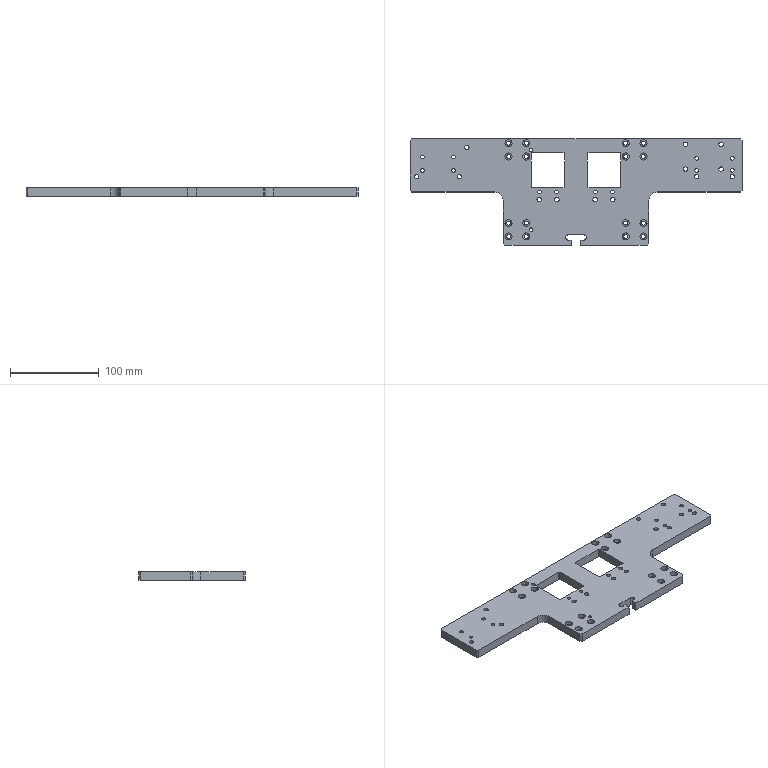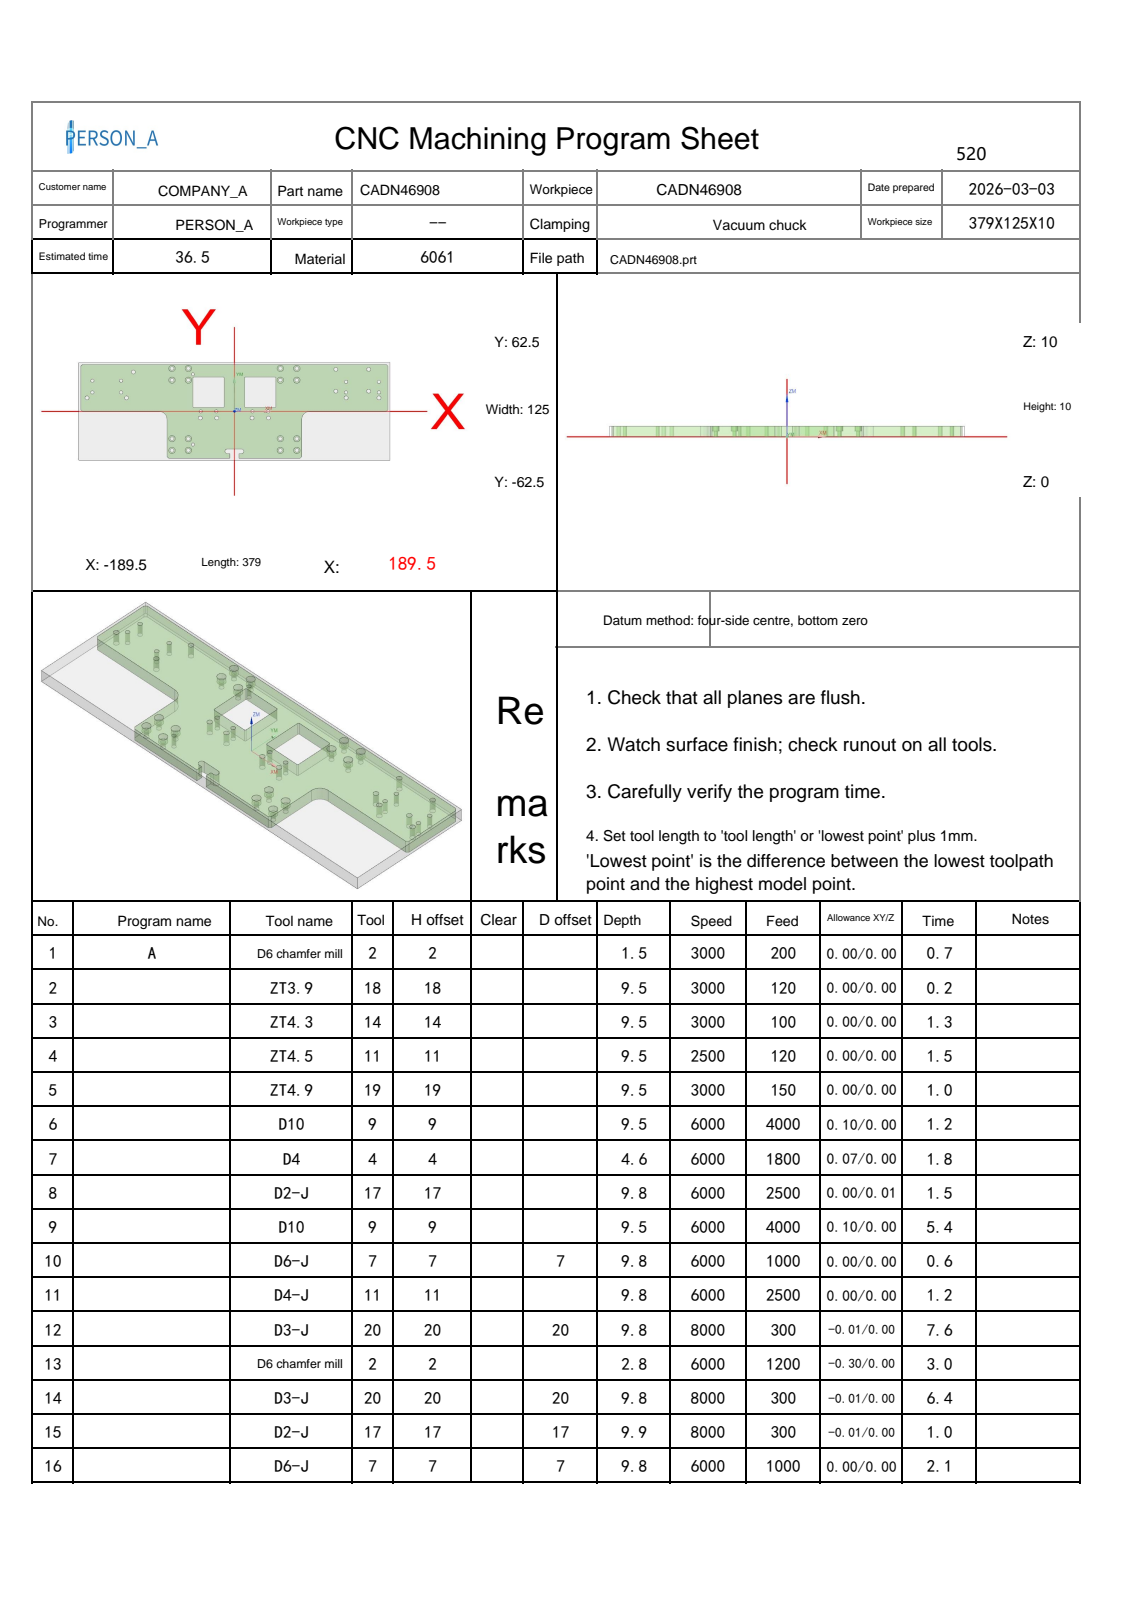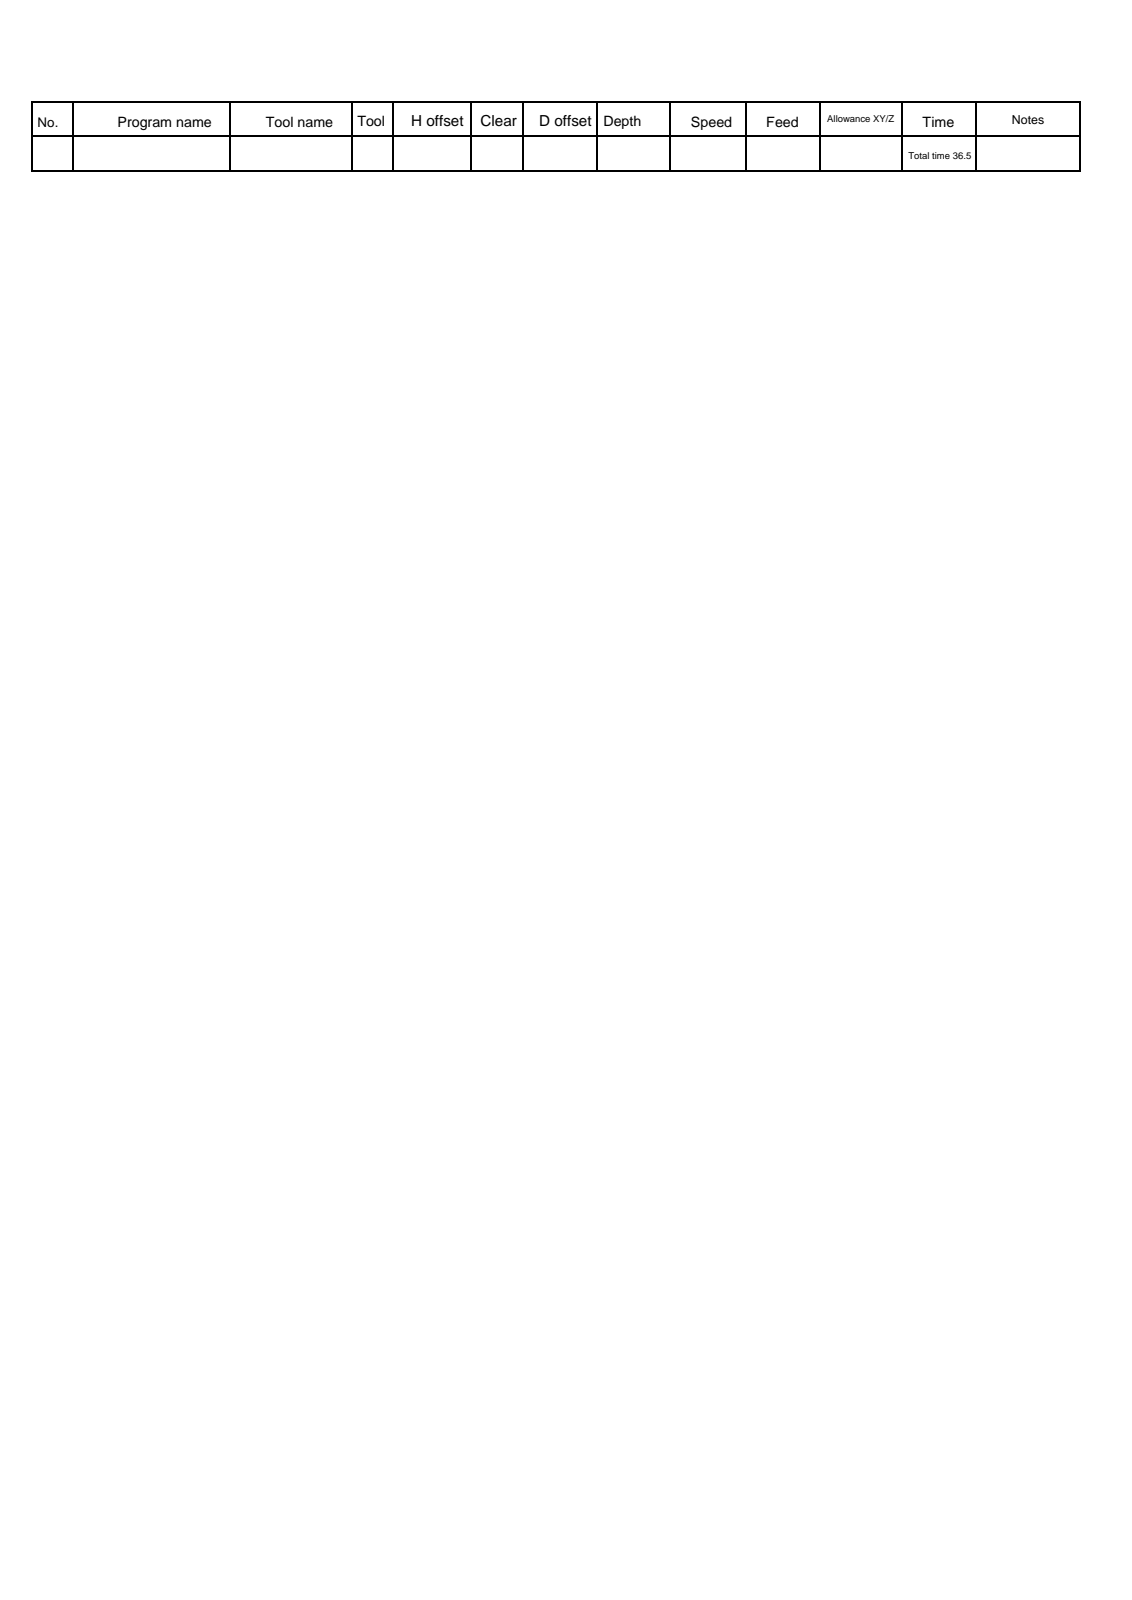NC program | NX | posted by the shop | part box 374 x 120 x 10 mm
Lines 7021 to 8155 of 15301:
N11 T11 M06
(D4-J  D=4. R=0. H=11 ce=0.00 di=0.00)
G00 G90 G54 X-76. Y55. M03 S6000
G43 H11 Z40.
M08
Z5.4
G01 X-74.404 Y54.671 F600.
X-74.336 Y54.664
G03 X-74. Y55. I0.0 J.336
X-76. Y57. I-2. J0.0
X-78. Y55. I0.0 J-2.
X-76. Y53. I2. J0.0
X-74. Y55. I0.0 J2.
X-74.062 Y55.495 I-2. J0.0
X-74.388 Y55.748 I-.325 J-.083
G01 X-74.535 Y55.714
X-76. Y55.
G00 Z40.
X-56.
Z5.4
G01 X-54.404 Y54.671
X-54.336 Y54.664
G03 X-54. Y55. I0.0 J.336
X-56. Y57. I-2. J0.0
X-58. Y55. I0.0 J-2.
X-56. Y53. I2. J0.0
X-54. Y55. I0.0 J2.
X-54.062 Y55.495 I-2. J0.0
X-54.388 Y55.748 I-.325 J-.083
G01 X-54.535 Y55.714
X-56. Y55.
G00 Z40.
Y40.
Z5.4
G01 X-54.404 Y39.671
X-54.336 Y39.664
G03 X-54. Y40. I0.0 J.336
X-56. Y42. I-2. J0.0
X-58. Y40. I0.0 J-2.
X-56. Y38. I2. J0.0
X-54. Y40. I0.0 J2.
X-54.062 Y40.495 I-2. J0.0
X-54.388 Y40.748 I-.325 J-.083
G01 X-54.535 Y40.714
X-56. Y40.
G00 Z40.
X-76.
Z5.4
G01 X-74.404 Y39.671
X-74.336 Y39.664
G03 X-74. Y40. I0.0 J.336
X-76. Y42. I-2. J0.0
X-78. Y40. I0.0 J-2.
X-76. Y38. I2. J0.0
X-74. Y40. I0.0 J2.
X-74.062 Y40.495 I-2. J0.0
X-74.388 Y40.748 I-.325 J-.083
G01 X-74.535 Y40.714
X-76. Y40.
G00 Z40.
Y-35.
Z5.4
G01 X-74.404 Y-35.329
X-74.336 Y-35.336
G03 X-74. Y-35. I0.0 J.336
X-76. Y-33. I-2. J0.0
X-78. Y-35. I0.0 J-2.
X-76. Y-37. I2. J0.0
X-74. Y-35. I0.0 J2.
X-74.062 Y-34.505 I-2. J0.0
X-74.388 Y-34.252 I-.325 J-.083
G01 X-74.535 Y-34.286
X-76. Y-35.
G00 Z40.
Y-50.
Z5.4
G01 X-74.404 Y-50.329
X-74.336 Y-50.336
G03 X-74. Y-50. I0.0 J.336
X-76. Y-48. I-2. J0.0
X-78. Y-50. I0.0 J-2.
X-76. Y-52. I2. J0.0
X-74. Y-50. I0.0 J2.
X-74.062 Y-49.505 I-2. J0.0
X-74.388 Y-49.252 I-.325 J-.083
G01 X-74.535 Y-49.286
X-76. Y-50.
G00 Z40.
X-56.
Z5.4
G01 X-54.404 Y-50.329
X-54.336 Y-50.336
G03 X-54. Y-50. I0.0 J.336
X-56. Y-48. I-2. J0.0
X-58. Y-50. I0.0 J-2.
X-56. Y-52. I2. J0.0
X-54. Y-50. I0.0 J2.
X-54.062 Y-49.505 I-2. J0.0
X-54.388 Y-49.252 I-.325 J-.083
G01 X-54.535 Y-49.286
X-56. Y-50.
G00 Z40.
Y-35.
Z5.4
G01 X-54.404 Y-35.329
X-54.336 Y-35.336
G03 X-54. Y-35. I0.0 J.336
X-56. Y-33. I-2. J0.0
X-58. Y-35. I0.0 J-2.
X-56. Y-37. I2. J0.0
X-54. Y-35. I0.0 J2.
X-54.062 Y-34.505 I-2. J0.0
X-54.388 Y-34.252 I-.325 J-.083
G01 X-54.535 Y-34.286
X-56. Y-35.
G00 Z40.
X56.
Z5.4
G01 X57.596 Y-35.329
X57.664 Y-35.336
G03 X58. Y-35. I0.0 J.336
X56. Y-33. I-2. J0.0
X54. Y-35. I0.0 J-2.
X56. Y-37. I2. J0.0
X58. Y-35. I0.0 J2.
X57.938 Y-34.505 I-2. J0.0
X57.612 Y-34.252 I-.325 J-.083
G01 X57.465 Y-34.286
X56. Y-35.
G00 Z40.
Y-50.
Z5.4
G01 X57.596 Y-50.329
X57.664 Y-50.336
G03 X58. Y-50. I0.0 J.336
X56. Y-48. I-2. J0.0
X54. Y-50. I0.0 J-2.
X56. Y-52. I2. J0.0
X58. Y-50. I0.0 J2.
X57.938 Y-49.505 I-2. J0.0
X57.612 Y-49.252 I-.325 J-.083
G01 X57.465 Y-49.286
X56. Y-50.
G00 Z40.
X76.
Z5.4
G01 X77.596 Y-50.329
X77.664 Y-50.336
G03 X78. Y-50. I0.0 J.336
X76. Y-48. I-2. J0.0
X74. Y-50. I0.0 J-2.
X76. Y-52. I2. J0.0
X78. Y-50. I0.0 J2.
X77.938 Y-49.505 I-2. J0.0
X77.612 Y-49.252 I-.325 J-.083
G01 X77.465 Y-49.286
X76. Y-50.
G00 Z40.
Y-35.
Z5.4
G01 X77.596 Y-35.329
X77.664 Y-35.336
G03 X78. Y-35. I0.0 J.336
X76. Y-33. I-2. J0.0
X74. Y-35. I0.0 J-2.
X76. Y-37. I2. J0.0
X78. Y-35. I0.0 J2.
X77.938 Y-34.505 I-2. J0.0
X77.612 Y-34.252 I-.325 J-.083
G01 X77.465 Y-34.286
X76. Y-35.
G00 Z40.
Y40.
Z5.4
G01 X77.596 Y39.671
X77.664 Y39.664
G03 X78. Y40. I0.0 J.336
X76. Y42. I-2. J0.0
X74. Y40. I0.0 J-2.
X76. Y38. I2. J0.0
X78. Y40. I0.0 J2.
X77.938 Y40.495 I-2. J0.0
X77.612 Y40.748 I-.325 J-.083
G01 X77.465 Y40.714
X76. Y40.
G00 Z40.
Y55.
Z5.4
G01 X77.596 Y54.671
X77.664 Y54.664
G03 X78. Y55. I0.0 J.336
X76. Y57. I-2. J0.0
X74. Y55. I0.0 J-2.
X76. Y53. I2. J0.0
X78. Y55. I0.0 J2.
X77.938 Y55.495 I-2. J0.0
X77.612 Y55.748 I-.325 J-.083
G01 X77.465 Y55.714
X76. Y55.
G00 Z40.
X56.
Z5.4
G01 X57.596 Y54.671
X57.664 Y54.664
G03 X58. Y55. I0.0 J.336
X56. Y57. I-2. J0.0
X54. Y55. I0.0 J-2.
X56. Y53. I2. J0.0
X58. Y55. I0.0 J2.
X57.938 Y55.495 I-2. J0.0
X57.612 Y55.748 I-.325 J-.083
G01 X57.465 Y55.714
X56. Y55.
G00 Z40.
Y40.
Z5.4
G01 X57.596 Y39.671
X57.664 Y39.664
G03 X58. Y40. I0.0 J.336
X56. Y42. I-2. J0.0
X54. Y40. I0.0 J-2.
X56. Y38. I2. J0.0
X58. Y40. I0.0 J2.
X57.938 Y40.495 I-2. J0.0
X57.612 Y40.748 I-.325 J-.083
G01 X57.465 Y40.714
X56. Y40.
G00 Z40.
G00 G90 X2.877 Y-54.442 M03 S6000
Z40.
Z10.303
G01 X2.884 Z10.217 F2000.
X2.904 Y-54.44 Z10.139
X2.934 Y-54.436 Z10.069
X2.973 Y-54.431 Z10.007
X3.019 Y-54.422 Z9.951
X3.07 Y-54.412 Z9.902
X3.126 Y-54.398 Z9.86
X3.183 Y-54.381 Z9.823
X3.241 Y-54.359 Z9.792
X3.297 Y-54.334 Z9.766
X3.35 Y-54.305 Z9.746
X3.398 Y-54.271 Z9.729
X3.439 Y-54.231 Z9.717
X3.471 Y-54.186 Z9.709
X3.493 Y-54.136 Z9.704
X3.504 Y-54.079 Z9.703
G02 X5.5 Y-52.2 I1.996 J-.121 F2500.
G01 X8.5
G03 X9.5 Y-51.2 I0.0 J1.
X8.5 Y-50.2 I-1. J0.0
G01 X.448
X.407 Y-50.215 Z9.702
X.384 Y-50.259 Z9.7
X.378 Y-50.329 Z9.697
X.386 Y-50.421 Z9.692
X.409 Y-50.533 Z9.686
X.445 Y-50.663 Z9.679
X.493 Y-50.806 Z9.671
X.586 Y-51.048 Z9.658
X.706 Y-51.316 Z9.642
X.864 Y-51.636 Z9.623
X1.095 Y-52.036 Z9.596
X1.351 Y-52.416 Z9.568
X1.632 Y-52.773 Z9.541
X1.936 Y-53.107 Z9.513
X2.265 Y-53.415 Z9.486
X2.497 Y-53.605 Z9.469
X2.734 Y-53.781 Z9.453
X2.884 Y-53.882 Z9.443
X3.026 Y-53.968 Z9.434
X3.155 Y-54.039 Z9.426
X3.269 Y-54.091 Z9.419
X3.364 Y-54.124 Z9.414
X3.437 Y-54.134 Z9.41
X3.485 Y-54.12 Z9.407
X3.504 Y-54.079 Z9.406
G02 X5.5 Y-52.2 I1.996 J-.121
G01 X8.5
G03 X9.5 Y-51.2 I0.0 J1.
X8.5 Y-50.2 I-1. J0.0
G01 X.448
X.407 Y-50.215 Z9.405
X.384 Y-50.259 Z9.403
X.378 Y-50.329 Z9.4
X.386 Y-50.421 Z9.395
X.409 Y-50.533 Z9.389
X.445 Y-50.663 Z9.382
X.493 Y-50.806 Z9.374
X.586 Y-51.048 Z9.361
X.706 Y-51.316 Z9.345
X.864 Y-51.636 Z9.326
X1.095 Y-52.036 Z9.299
X1.351 Y-52.416 Z9.271
X1.632 Y-52.773 Z9.244
X1.936 Y-53.107 Z9.216
X2.265 Y-53.415 Z9.19
X2.497 Y-53.605 Z9.172
X2.734 Y-53.781 Z9.156
X2.884 Y-53.882 Z9.146
X3.026 Y-53.968 Z9.137
X3.155 Y-54.039 Z9.129
X3.269 Y-54.091 Z9.122
X3.364 Y-54.124 Z9.117
X3.437 Y-54.134 Z9.113
X3.485 Y-54.12 Z9.11
X3.504 Y-54.079 Z9.109
G02 X5.5 Y-52.2 I1.996 J-.121
G01 X8.5
G03 X9.5 Y-51.2 I0.0 J1.
X8.5 Y-50.2 I-1. J0.0
G01 X.448
X.407 Y-50.215 Z9.108
X.384 Y-50.259 Z9.106
X.378 Y-50.329 Z9.103
X.386 Y-50.421 Z9.098
X.409 Y-50.533 Z9.092
X.445 Y-50.663 Z9.085
X.493 Y-50.806 Z9.077
X.586 Y-51.048 Z9.064
X.706 Y-51.316 Z9.048
X.864 Y-51.636 Z9.029
X1.095 Y-52.036 Z9.002
X1.351 Y-52.416 Z8.975
X1.632 Y-52.773 Z8.947
X1.936 Y-53.107 Z8.919
X2.265 Y-53.415 Z8.893
X2.497 Y-53.605 Z8.875
X2.734 Y-53.781 Z8.859
X2.884 Y-53.882 Z8.849
X3.026 Y-53.968 Z8.84
X3.155 Y-54.039 Z8.832
X3.269 Y-54.091 Z8.825
X3.364 Y-54.124 Z8.82
X3.437 Y-54.134 Z8.816
X3.485 Y-54.12 Z8.813
X3.504 Y-54.079 Z8.812
G02 X5.5 Y-52.2 I1.996 J-.121
G01 X8.5
G03 X9.5 Y-51.2 I0.0 J1.
X8.5 Y-50.2 I-1. J0.0
G01 X.448
X.407 Y-50.215 Z8.811
X.384 Y-50.259 Z8.809
X.378 Y-50.329 Z8.806
X.386 Y-50.421 Z8.801
X.409 Y-50.533 Z8.795
X.445 Y-50.663 Z8.788
X.493 Y-50.806 Z8.78
X.586 Y-51.048 Z8.767
X.706 Y-51.316 Z8.751
X.864 Y-51.636 Z8.732
X1.095 Y-52.036 Z8.705
X1.351 Y-52.416 Z8.678
X1.632 Y-52.773 Z8.65
X1.936 Y-53.107 Z8.622
X2.265 Y-53.415 Z8.596
X2.497 Y-53.605 Z8.579
X2.734 Y-53.781 Z8.562
X2.884 Y-53.882 Z8.552
X3.026 Y-53.968 Z8.543
X3.155 Y-54.039 Z8.535
X3.269 Y-54.091 Z8.528
X3.364 Y-54.124 Z8.523
X3.437 Y-54.134 Z8.519
X3.485 Y-54.12 Z8.516
X3.504 Y-54.079 Z8.515
G02 X5.5 Y-52.2 I1.996 J-.121
G01 X8.5
G03 X9.5 Y-51.2 I0.0 J1.
X8.5 Y-50.2 I-1. J0.0
G01 X.448
X.407 Y-50.215 Z8.514
X.384 Y-50.259 Z8.512
X.378 Y-50.329 Z8.509
X.386 Y-50.421 Z8.504
X.409 Y-50.533 Z8.498
X.445 Y-50.663 Z8.491
X.493 Y-50.806 Z8.483
X.586 Y-51.048 Z8.47
X.706 Y-51.316 Z8.454
X.864 Y-51.636 Z8.435
X1.095 Y-52.036 Z8.408
X1.351 Y-52.416 Z8.381
X1.632 Y-52.773 Z8.353
X1.936 Y-53.107 Z8.325
X2.265 Y-53.415 Z8.299
X2.497 Y-53.605 Z8.282
X2.734 Y-53.781 Z8.265
X2.884 Y-53.882 Z8.255
X3.026 Y-53.968 Z8.246
X3.155 Y-54.039 Z8.238
X3.269 Y-54.091 Z8.231
X3.364 Y-54.124 Z8.226
X3.437 Y-54.134 Z8.222
X3.485 Y-54.12 Z8.219
X3.504 Y-54.079 Z8.218
G02 X5.5 Y-52.2 I1.996 J-.121
G01 X8.5
G03 X9.5 Y-51.2 I0.0 J1.
X8.5 Y-50.2 I-1. J0.0
G01 X.448
X.407 Y-50.215 Z8.217
X.384 Y-50.259 Z8.215
X.378 Y-50.329 Z8.212
X.386 Y-50.421 Z8.207
X.409 Y-50.533 Z8.201
X.445 Y-50.663 Z8.194
X.493 Y-50.806 Z8.186
X.586 Y-51.048 Z8.173
X.706 Y-51.316 Z8.157
X.864 Y-51.636 Z8.138
X1.095 Y-52.036 Z8.111
X1.351 Y-52.416 Z8.084
X1.632 Y-52.773 Z8.056
X1.936 Y-53.107 Z8.028
X2.265 Y-53.415 Z8.002
X2.497 Y-53.605 Z7.985
X2.734 Y-53.781 Z7.968
X2.884 Y-53.882 Z7.958
X3.026 Y-53.968 Z7.949
X3.155 Y-54.039 Z7.941
X3.269 Y-54.091 Z7.934
X3.364 Y-54.124 Z7.929
X3.437 Y-54.134 Z7.925
X3.485 Y-54.12 Z7.922
X3.504 Y-54.079 Z7.921
G02 X5.5 Y-52.2 I1.996 J-.121
G01 X8.5
G03 X9.5 Y-51.2 I0.0 J1.
X8.5 Y-50.2 I-1. J0.0
G01 X.448
X.407 Y-50.215 Z7.92
X.384 Y-50.259 Z7.918
X.378 Y-50.329 Z7.915
X.386 Y-50.421 Z7.91
X.409 Y-50.533 Z7.904
X.445 Y-50.663 Z7.897
X.493 Y-50.806 Z7.889
X.586 Y-51.048 Z7.876
X.706 Y-51.316 Z7.86
X.864 Y-51.636 Z7.841
X1.095 Y-52.036 Z7.814
X1.351 Y-52.416 Z7.787
X1.632 Y-52.773 Z7.759
X1.936 Y-53.107 Z7.731
X2.265 Y-53.415 Z7.705
X2.497 Y-53.605 Z7.688
X2.734 Y-53.781 Z7.671
X2.884 Y-53.882 Z7.661
X3.026 Y-53.968 Z7.652
X3.155 Y-54.039 Z7.644
X3.269 Y-54.091 Z7.637
X3.364 Y-54.124 Z7.632
X3.437 Y-54.134 Z7.628
X3.485 Y-54.12 Z7.625
X3.504 Y-54.079 Z7.624
G02 X5.5 Y-52.2 I1.996 J-.121
G01 X8.5
G03 X9.5 Y-51.2 I0.0 J1.
X8.5 Y-50.2 I-1. J0.0
G01 X.448
X.407 Y-50.215 Z7.623
X.384 Y-50.259 Z7.621
X.378 Y-50.329 Z7.618
X.386 Y-50.421 Z7.613
X.409 Y-50.533 Z7.607
X.445 Y-50.663 Z7.6
X.493 Y-50.806 Z7.592
X.586 Y-51.048 Z7.579
X.706 Y-51.316 Z7.563
X.864 Y-51.636 Z7.544
X1.095 Y-52.036 Z7.517
X1.351 Y-52.416 Z7.49
X1.632 Y-52.773 Z7.462
X1.936 Y-53.107 Z7.434
X2.265 Y-53.415 Z7.408
X2.497 Y-53.605 Z7.391
X2.734 Y-53.781 Z7.374
X2.884 Y-53.882 Z7.364
X3.026 Y-53.968 Z7.355
X3.155 Y-54.039 Z7.347
X3.269 Y-54.091 Z7.341
X3.364 Y-54.124 Z7.335
X3.437 Y-54.134 Z7.331
X3.485 Y-54.12 Z7.328
X3.504 Y-54.079 Z7.327
G02 X5.5 Y-52.2 I1.996 J-.121
G01 X8.5
G03 X9.5 Y-51.2 I0.0 J1.
X8.5 Y-50.2 I-1. J0.0
G01 X.448
X.407 Y-50.215
X.384 Y-50.259 Z7.324
X.378 Y-50.329 Z7.321
X.386 Y-50.421 Z7.316
X.409 Y-50.533 Z7.31
X.445 Y-50.663 Z7.303
X.493 Y-50.806 Z7.296
X.586 Y-51.048 Z7.282
X.706 Y-51.316 Z7.266
X.864 Y-51.636 Z7.247
X1.095 Y-52.036 Z7.22
X1.351 Y-52.416 Z7.193
X1.632 Y-52.773 Z7.165
X1.936 Y-53.107 Z7.137
X2.265 Y-53.415 Z7.111
X2.497 Y-53.605 Z7.094
X2.734 Y-53.781 Z7.077
X2.884 Y-53.882 Z7.067
X3.026 Y-53.968 Z7.058
X3.155 Y-54.039 Z7.05
X3.269 Y-54.091 Z7.044
X3.364 Y-54.124 Z7.038
X3.437 Y-54.134 Z7.034
X3.485 Y-54.12 Z7.031
X3.504 Y-54.079 Z7.03
G02 X5.5 Y-52.2 I1.996 J-.121
G01 X8.5
G03 X9.5 Y-51.2 I0.0 J1.
X8.5 Y-50.2 I-1. J0.0
G01 X.448
X.407 Y-50.215
X.384 Y-50.259 Z7.027
X.378 Y-50.329 Z7.024
X.386 Y-50.421 Z7.019
X.409 Y-50.533 Z7.013
X.445 Y-50.663 Z7.006
X.493 Y-50.806 Z6.999
X.586 Y-51.048 Z6.985
X.706 Y-51.316 Z6.969
X.864 Y-51.636 Z6.95
X1.095 Y-52.036 Z6.923
X1.351 Y-52.416 Z6.896
X1.632 Y-52.773 Z6.868
X1.936 Y-53.107 Z6.84
X2.265 Y-53.415 Z6.814
X2.497 Y-53.605 Z6.797
X2.734 Y-53.781 Z6.78
X2.884 Y-53.882 Z6.77
X3.026 Y-53.968 Z6.761
X3.155 Y-54.039 Z6.753
X3.269 Y-54.091 Z6.747
X3.364 Y-54.124 Z6.741
X3.437 Y-54.134 Z6.737
X3.485 Y-54.12 Z6.734
X3.504 Y-54.079 Z6.733
G02 X5.5 Y-52.2 I1.996 J-.121
G01 X8.5
G03 X9.5 Y-51.2 I0.0 J1.
X8.5 Y-50.2 I-1. J0.0
G01 X.448
X.407 Y-50.215
X.384 Y-50.259 Z6.73
X.378 Y-50.329 Z6.727
X.386 Y-50.421 Z6.722
X.409 Y-50.533 Z6.716
X.445 Y-50.663 Z6.709
X.493 Y-50.806 Z6.702
X.586 Y-51.048 Z6.688
X.706 Y-51.316 Z6.672
X.864 Y-51.636 Z6.653
X1.095 Y-52.036 Z6.626
X1.351 Y-52.416 Z6.599
X1.632 Y-52.773 Z6.571
X1.936 Y-53.107 Z6.543
X2.265 Y-53.415 Z6.517
X2.497 Y-53.605 Z6.5
X2.734 Y-53.781 Z6.483
X2.884 Y-53.882 Z6.473
X3.026 Y-53.968 Z6.464
X3.155 Y-54.039 Z6.456
X3.269 Y-54.091 Z6.45
X3.364 Y-54.124 Z6.444
X3.437 Y-54.134 Z6.44
X3.485 Y-54.12 Z6.437
X3.504 Y-54.079 Z6.436
G02 X5.5 Y-52.2 I1.996 J-.121
G01 X8.5
G03 X9.5 Y-51.2 I0.0 J1.
X8.5 Y-50.2 I-1. J0.0
G01 X.448
X.407 Y-50.215
X.384 Y-50.259 Z6.433
X.378 Y-50.329 Z6.43
X.386 Y-50.421 Z6.425
X.409 Y-50.533 Z6.419
X.445 Y-50.663 Z6.412
X.493 Y-50.806 Z6.405
X.586 Y-51.048 Z6.391
X.706 Y-51.316 Z6.376
X.864 Y-51.636 Z6.356
X1.095 Y-52.036 Z6.329
X1.351 Y-52.416 Z6.302
X1.632 Y-52.773 Z6.274
X1.936 Y-53.107 Z6.246
X2.265 Y-53.415 Z6.22
X2.497 Y-53.605 Z6.203
X2.734 Y-53.781 Z6.186
X2.884 Y-53.882 Z6.177
X3.026 Y-53.968 Z6.168
X3.155 Y-54.039 Z6.159
X3.269 Y-54.091 Z6.153
X3.364 Y-54.124 Z6.147
X3.437 Y-54.134 Z6.143
X3.485 Y-54.12 Z6.14
X3.504 Y-54.079 Z6.139
G02 X5.5 Y-52.2 I1.996 J-.121
G01 X8.5
G03 X9.5 Y-51.2 I0.0 J1.
X8.5 Y-50.2 I-1. J0.0
G01 X.448
X.407 Y-50.215
X.384 Y-50.259 Z6.136
X.378 Y-50.329 Z6.133
X.386 Y-50.421 Z6.128
X.409 Y-50.533 Z6.122
X.445 Y-50.663 Z6.115
X.493 Y-50.806 Z6.108
X.586 Y-51.048 Z6.094
X.706 Y-51.316 Z6.079
X.864 Y-51.636 Z6.059
X1.095 Y-52.036 Z6.032
X1.351 Y-52.416 Z6.005
X1.632 Y-52.773 Z5.977
X1.936 Y-53.107 Z5.949
X2.265 Y-53.415 Z5.923
X2.497 Y-53.605 Z5.906
X2.734 Y-53.781 Z5.889
X2.884 Y-53.882 Z5.88
X3.026 Y-53.968 Z5.871
X3.155 Y-54.039 Z5.863
X3.269 Y-54.091 Z5.856
X3.364 Y-54.124 Z5.85
X3.437 Y-54.134 Z5.846
X3.485 Y-54.12 Z5.843
X3.504 Y-54.079 Z5.842
G02 X5.5 Y-52.2 I1.996 J-.121
G01 X8.5
G03 X9.5 Y-51.2 I0.0 J1.
X8.5 Y-50.2 I-1. J0.0
G01 X.448
X.407 Y-50.215
X.384 Y-50.259 Z5.839
X.378 Y-50.329 Z5.836
X.386 Y-50.421 Z5.831
X.409 Y-50.533 Z5.825
X.445 Y-50.663 Z5.818
X.493 Y-50.806 Z5.811
X.586 Y-51.048 Z5.797
X.706 Y-51.316 Z5.782
X.864 Y-51.636 Z5.762
X1.095 Y-52.036 Z5.735
X1.351 Y-52.416 Z5.708
X1.632 Y-52.773 Z5.68
X1.936 Y-53.107 Z5.653
X2.265 Y-53.415 Z5.626
X2.497 Y-53.605 Z5.609
X2.734 Y-53.781 Z5.592
X2.884 Y-53.882 Z5.583
X3.026 Y-53.968 Z5.574
X3.155 Y-54.039 Z5.566
X3.269 Y-54.091 Z5.559
X3.364 Y-54.124 Z5.553
X3.437 Y-54.134 Z5.549
X3.485 Y-54.12 Z5.546
X3.504 Y-54.079 Z5.545
G02 X5.5 Y-52.2 I1.996 J-.121
G01 X8.5
G03 X9.5 Y-51.2 I0.0 J1.
X8.5 Y-50.2 I-1. J0.0
G01 X.448
X.407 Y-50.215
X.384 Y-50.259 Z5.543
X.378 Y-50.329 Z5.539
X.386 Y-50.421 Z5.534
X.409 Y-50.533 Z5.528
X.445 Y-50.663 Z5.521
X.493 Y-50.806 Z5.514
X.586 Y-51.048 Z5.5
X.706 Y-51.316 Z5.485
X.864 Y-51.636 Z5.465
X1.095 Y-52.036 Z5.438
X1.351 Y-52.416 Z5.411
X1.632 Y-52.773 Z5.383
X1.936 Y-53.107 Z5.356
X2.265 Y-53.415 Z5.329
X2.497 Y-53.605 Z5.312
X2.734 Y-53.781 Z5.295
X2.884 Y-53.882 Z5.286
X3.026 Y-53.968 Z5.277
X3.155 Y-54.039 Z5.269
X3.269 Y-54.091 Z5.262
X3.364 Y-54.124 Z5.256
X3.437 Y-54.134 Z5.252
X3.485 Y-54.12 Z5.249
X3.504 Y-54.079 Z5.248
G02 X5.5 Y-52.2 I1.996 J-.121
G01 X8.5
G03 X9.5 Y-51.2 I0.0 J1.
X8.5 Y-50.2 I-1. J0.0
G01 X.448
X.407 Y-50.215
X.384 Y-50.259 Z5.246
X.378 Y-50.329 Z5.242
X.386 Y-50.421 Z5.237
X.409 Y-50.533 Z5.231
X.445 Y-50.663 Z5.225
X.493 Y-50.806 Z5.217
X.586 Y-51.048 Z5.203
X.706 Y-51.316 Z5.188
X.864 Y-51.636 Z5.168
X1.095 Y-52.036 Z5.141
X1.351 Y-52.416 Z5.114
X1.632 Y-52.773 Z5.086
X1.936 Y-53.107 Z5.059
X2.265 Y-53.415 Z5.032
X2.497 Y-53.605 Z5.015
X2.734 Y-53.781 Z4.999
X2.884 Y-53.882 Z4.989
X3.026 Y-53.968 Z4.98
X3.155 Y-54.039 Z4.972
X3.269 Y-54.091 Z4.965
X3.364 Y-54.124 Z4.959
X3.437 Y-54.134 Z4.955
X3.485 Y-54.12 Z4.952
X3.504 Y-54.079
G02 X5.5 Y-52.2 I1.996 J-.121
G01 X8.5
G03 X9.5 Y-51.2 I0.0 J1.
X8.5 Y-50.2 I-1. J0.0
G01 X.448
X.407 Y-50.215 Z4.951
X.384 Y-50.259 Z4.949
X.378 Y-50.329 Z4.945
X.386 Y-50.421 Z4.94
X.409 Y-50.533 Z4.934
X.445 Y-50.663 Z4.928
X.493 Y-50.806 Z4.92
X.586 Y-51.048 Z4.906
X.706 Y-51.316 Z4.891
X.864 Y-51.636 Z4.871
X1.095 Y-52.036 Z4.844
X1.351 Y-52.416 Z4.817
X1.632 Y-52.773 Z4.789
X1.936 Y-53.107 Z4.762
X2.265 Y-53.415 Z4.735
X2.497 Y-53.605 Z4.718
X2.734 Y-53.781 Z4.702
X2.884 Y-53.882 Z4.692
X3.026 Y-53.968 Z4.683
X3.155 Y-54.039 Z4.675
X3.269 Y-54.091 Z4.668
X3.364 Y-54.124 Z4.662
X3.437 Y-54.134 Z4.658
X3.485 Y-54.12 Z4.655
X3.504 Y-54.079
G02 X5.5 Y-52.2 I1.996 J-.121
G01 X8.5
G03 X9.5 Y-51.2 I0.0 J1.
X8.5 Y-50.2 I-1. J0.0
G01 X.448
X.407 Y-50.215 Z4.654
X.384 Y-50.259 Z4.652
X.378 Y-50.329 Z4.648
X.386 Y-50.421 Z4.643
X.409 Y-50.533 Z4.637
X.445 Y-50.663 Z4.631
X.493 Y-50.806 Z4.623
X.586 Y-51.048 Z4.609
X.706 Y-51.316 Z4.594
X.864 Y-51.636 Z4.574
X1.095 Y-52.036 Z4.547
X1.351 Y-52.416 Z4.52
X1.632 Y-52.773 Z4.492
X1.936 Y-53.107 Z4.465
X2.265 Y-53.415 Z4.438
X2.497 Y-53.605 Z4.421
X2.734 Y-53.781 Z4.405
X2.884 Y-53.882 Z4.395
X3.026 Y-53.968 Z4.386
X3.155 Y-54.039 Z4.378
X3.269 Y-54.091 Z4.371
X3.364 Y-54.124 Z4.365
X3.437 Y-54.134 Z4.361
X3.485 Y-54.12 Z4.358
X3.504 Y-54.079
G02 X5.5 Y-52.2 I1.996 J-.121
G01 X8.5
G03 X9.5 Y-51.2 I0.0 J1.
X8.5 Y-50.2 I-1. J0.0
G01 X.448
X.407 Y-50.215 Z4.357
X.384 Y-50.259 Z4.355
X.378 Y-50.329 Z4.351
X.386 Y-50.421 Z4.346
X.409 Y-50.533 Z4.34
X.445 Y-50.663 Z4.334
X.493 Y-50.806 Z4.326
X.586 Y-51.048 Z4.312
X.706 Y-51.316 Z4.297
X.864 Y-51.636 Z4.277
X1.095 Y-52.036 Z4.251
X1.351 Y-52.416 Z4.223
X1.632 Y-52.773 Z4.195
X1.936 Y-53.107 Z4.168
X2.265 Y-53.415 Z4.141
X2.497 Y-53.605 Z4.124
X2.734 Y-53.781 Z4.108
X2.884 Y-53.882 Z4.098
X3.026 Y-53.968 Z4.089
X3.155 Y-54.039 Z4.081
X3.269 Y-54.091 Z4.074
X3.364 Y-54.124 Z4.068
X3.437 Y-54.134 Z4.064
X3.485 Y-54.12 Z4.062
X3.504 Y-54.079 Z4.061
G02 X5.5 Y-52.2 I1.996 J-.121
G01 X8.5
G03 X9.5 Y-51.2 I0.0 J1.
X8.5 Y-50.2 I-1. J0.0
G01 X.448
X.407 Y-50.215 Z4.06
X.384 Y-50.259 Z4.058
X.378 Y-50.329 Z4.054
X.386 Y-50.421 Z4.049
X.409 Y-50.533 Z4.044
X.445 Y-50.663 Z4.037
X.493 Y-50.806 Z4.029
X.586 Y-51.048 Z4.015
X.706 Y-51.316 Z4.
X.864 Y-51.636 Z3.98
X1.095 Y-52.036 Z3.954
X1.351 Y-52.416 Z3.926
X1.632 Y-52.773 Z3.898
X1.936 Y-53.107 Z3.871
X2.265 Y-53.415 Z3.844
X2.497 Y-53.605 Z3.827
X2.734 Y-53.781 Z3.811
X2.884 Y-53.882 Z3.801
X3.026 Y-53.968 Z3.792
X3.155 Y-54.039 Z3.784
X3.269 Y-54.091 Z3.777
X3.364 Y-54.124 Z3.771
X3.437 Y-54.134 Z3.767
X3.485 Y-54.12 Z3.765
X3.504 Y-54.079 Z3.764
G02 X5.5 Y-52.2 I1.996 J-.121
G01 X8.5
G03 X9.5 Y-51.2 I0.0 J1.
X8.5 Y-50.2 I-1. J0.0
G01 X.448
X.407 Y-50.215 Z3.763
X.384 Y-50.259 Z3.761
X.378 Y-50.329 Z3.757
X.386 Y-50.421 Z3.752
X.409 Y-50.533 Z3.747
X.445 Y-50.663 Z3.74
X.493 Y-50.806 Z3.732
X.586 Y-51.048 Z3.718
X.706 Y-51.316 Z3.703
X.864 Y-51.636 Z3.683
X1.095 Y-52.036 Z3.657
X1.351 Y-52.416 Z3.629
X1.632 Y-52.773 Z3.601
X1.936 Y-53.107 Z3.574
X2.265 Y-53.415 Z3.547
X2.497 Y-53.605 Z3.53
X2.734 Y-53.781 Z3.514
X2.884 Y-53.882 Z3.504
X3.026 Y-53.968 Z3.495
X3.155 Y-54.039 Z3.487
X3.269 Y-54.091 Z3.48
X3.364 Y-54.124 Z3.474
X3.437 Y-54.134 Z3.47
X3.485 Y-54.12 Z3.468
X3.504 Y-54.079 Z3.467
G02 X5.5 Y-52.2 I1.996 J-.121
G01 X8.5
G03 X9.5 Y-51.2 I0.0 J1.
X8.5 Y-50.2 I-1. J0.0
G01 X.448
X.407 Y-50.215 Z3.466
X.384 Y-50.259 Z3.464
X.378 Y-50.329 Z3.46
X.386 Y-50.421 Z3.455
X.409 Y-50.533 Z3.45
X.445 Y-50.663 Z3.443
X.493 Y-50.806 Z3.435
X.586 Y-51.048 Z3.421
X.706 Y-51.316 Z3.406
X.864 Y-51.636 Z3.386
X1.095 Y-52.036 Z3.36
X1.351 Y-52.416 Z3.332
X1.632 Y-52.773 Z3.304
X1.936 Y-53.107 Z3.277
X2.265 Y-53.415 Z3.25
X2.497 Y-53.605 Z3.233
X2.734 Y-53.781 Z3.217
X2.884 Y-53.882 Z3.207
X3.026 Y-53.968 Z3.198
X3.155 Y-54.039 Z3.19
X3.269 Y-54.091 Z3.183
X3.364 Y-54.124 Z3.177
X3.437 Y-54.134 Z3.173
X3.485 Y-54.12 Z3.171
X3.504 Y-54.079 Z3.17
G02 X5.5 Y-52.2 I1.996 J-.121
G01 X8.5
G03 X9.5 Y-51.2 I0.0 J1.
X8.5 Y-50.2 I-1. J0.0
G01 X.448
X.407 Y-50.215 Z3.169
X.384 Y-50.259 Z3.167
X.378 Y-50.329 Z3.163
X.386 Y-50.421 Z3.158
X.409 Y-50.533 Z3.153
X.445 Y-50.663 Z3.146
X.493 Y-50.806 Z3.138
X.586 Y-51.048 Z3.124
X.706 Y-51.316 Z3.109
X.864 Y-51.636 Z3.089
X1.095 Y-52.036 Z3.063
X1.351 Y-52.416 Z3.035
X1.632 Y-52.773 Z3.007
X1.936 Y-53.107 Z2.98
X2.265 Y-53.415 Z2.953
X2.497 Y-53.605 Z2.936
X2.734 Y-53.781 Z2.92
X2.884 Y-53.882 Z2.91
X3.026 Y-53.968 Z2.901
X3.155 Y-54.039 Z2.893
X3.269 Y-54.091 Z2.886
X3.364 Y-54.124 Z2.88
X3.437 Y-54.134 Z2.876
X3.485 Y-54.12 Z2.874
X3.504 Y-54.079 Z2.873
G02 X5.5 Y-52.2 I1.996 J-.121
G01 X8.5
G03 X9.5 Y-51.2 I0.0 J1.
X8.5 Y-50.2 I-1. J0.0
G01 X.448
X.407 Y-50.215 Z2.872
X.384 Y-50.259 Z2.87
X.378 Y-50.329 Z2.866
X.386 Y-50.421 Z2.862
X.409 Y-50.533 Z2.856
X.445 Y-50.663 Z2.849
X.493 Y-50.806 Z2.841
X.586 Y-51.048 Z2.828
X.706 Y-51.316 Z2.812
X.864 Y-51.636 Z2.792
X1.095 Y-52.036 Z2.766
X1.351 Y-52.416 Z2.738
X1.632 Y-52.773 Z2.71
X1.936 Y-53.107 Z2.683
X2.265 Y-53.415 Z2.656
X2.497 Y-53.605 Z2.639
X2.734 Y-53.781 Z2.623
X2.884 Y-53.882 Z2.613
X3.026 Y-53.968 Z2.604
X3.155 Y-54.039 Z2.596
X3.269 Y-54.091 Z2.589
X3.364 Y-54.124 Z2.583
X3.437 Y-54.134 Z2.579
X3.485 Y-54.12 Z2.577
X3.504 Y-54.079 Z2.576
G02 X5.5 Y-52.2 I1.996 J-.121
G01 X8.5
G03 X9.5 Y-51.2 I0.0 J1.
X8.5 Y-50.2 I-1. J0.0
G01 X.448
X.407 Y-50.215 Z2.575
X.384 Y-50.259 Z2.573
X.378 Y-50.329 Z2.569
X.386 Y-50.421 Z2.565
X.409 Y-50.533 Z2.559
X.445 Y-50.663 Z2.552
X.493 Y-50.806 Z2.544
X.586 Y-51.048 Z2.531
X.706 Y-51.316 Z2.515
X.864 Y-51.636 Z2.495
X1.095 Y-52.036 Z2.469
X1.351 Y-52.416 Z2.441
X1.632 Y-52.773 Z2.413
X1.936 Y-53.107 Z2.386
X2.265 Y-53.415 Z2.359
X2.497 Y-53.605 Z2.342
X2.734 Y-53.781 Z2.326
X2.884 Y-53.882 Z2.316
X3.026 Y-53.968 Z2.307
X3.155 Y-54.039 Z2.299
X3.269 Y-54.091 Z2.292
X3.364 Y-54.124 Z2.286
X3.437 Y-54.134 Z2.282
X3.485 Y-54.12 Z2.28
X3.504 Y-54.079 Z2.279
G02 X5.5 Y-52.2 I1.996 J-.121
G01 X8.5
G03 X9.5 Y-51.2 I0.0 J1.
X8.5 Y-50.2 I-1. J0.0
G01 X.448
X.407 Y-50.215 Z2.278
X.384 Y-50.259 Z2.276
X.378 Y-50.329 Z2.272
X.386 Y-50.421 Z2.268
X.409 Y-50.533 Z2.262
X.445 Y-50.663 Z2.255
X.493 Y-50.806 Z2.247
X.586 Y-51.048 Z2.234
X.706 Y-51.316 Z2.218
X.864 Y-51.636 Z2.198
X1.095 Y-52.036 Z2.172
X1.351 Y-52.416 Z2.144
X1.632 Y-52.773 Z2.116
X1.936 Y-53.107 Z2.089
X2.265 Y-53.415 Z2.062
X2.497 Y-53.605 Z2.045
X2.734 Y-53.781 Z2.029
X2.884 Y-53.882 Z2.019
X3.026 Y-53.968 Z2.01
X3.155 Y-54.039 Z2.002
X3.269 Y-54.091 Z1.995
X3.364 Y-54.124 Z1.989
X3.437 Y-54.134 Z1.985
X3.485 Y-54.12 Z1.983
X3.504 Y-54.079 Z1.982
G02 X5.5 Y-52.2 I1.996 J-.121
G01 X8.5
G03 X9.5 Y-51.2 I0.0 J1.
X8.5 Y-50.2 I-1. J0.0
G01 X.448
X.407 Y-50.215 Z1.981
X.384 Y-50.259 Z1.979
X.378 Y-50.329 Z1.975
X.386 Y-50.421 Z1.971
X.409 Y-50.533 Z1.965
X.445 Y-50.663 Z1.958
X.493 Y-50.806 Z1.95
X.586 Y-51.048 Z1.937
X.706 Y-51.316 Z1.921
X.864 Y-51.636 Z1.901
X1.095 Y-52.036 Z1.875
X1.351 Y-52.416 Z1.847
X1.632 Y-52.773 Z1.819
X1.936 Y-53.107 Z1.792
X2.265 Y-53.415 Z1.765
X2.497 Y-53.605 Z1.748
X2.734 Y-53.781 Z1.732
X2.884 Y-53.882 Z1.722
X3.026 Y-53.968 Z1.713
X3.155 Y-54.039 Z1.705
X3.269 Y-54.091 Z1.698
X3.364 Y-54.124 Z1.693
X3.437 Y-54.134 Z1.688
X3.485 Y-54.12 Z1.686
X3.504 Y-54.079 Z1.685
G02 X5.5 Y-52.2 I1.996 J-.121
G01 X8.5
G03 X9.5 Y-51.2 I0.0 J1.
X8.5 Y-50.2 I-1. J0.0
G01 X.448
X.407 Y-50.215 Z1.684
X.384 Y-50.259 Z1.682
X.378 Y-50.329 Z1.678
X.386 Y-50.421 Z1.674
X.409 Y-50.533 Z1.668
X.445 Y-50.663 Z1.661
X.493 Y-50.806 Z1.653
X.586 Y-51.048 Z1.64
X.706 Y-51.316 Z1.624
X.864 Y-51.636 Z1.604
X1.095 Y-52.036 Z1.578
X1.351 Y-52.416 Z1.55
X1.632 Y-52.773 Z1.522
X1.936 Y-53.107 Z1.495
X2.265 Y-53.415 Z1.468
X2.497 Y-53.605 Z1.451
X2.734 Y-53.781 Z1.435
X2.884 Y-53.882 Z1.425
X3.026 Y-53.968 Z1.416
X3.155 Y-54.039 Z1.408
X3.269 Y-54.091 Z1.401
X3.364 Y-54.124 Z1.396
X3.437 Y-54.134 Z1.391
X3.485 Y-54.12 Z1.389
X3.504 Y-54.079 Z1.388
G02 X5.5 Y-52.2 I1.996 J-.121
G01 X8.5
G03 X9.5 Y-51.2 I0.0 J1.
X8.5 Y-50.2 I-1. J0.0
G01 X.448
X.407 Y-50.215 Z1.387
X.384 Y-50.259 Z1.385
X.378 Y-50.329 Z1.381
X.386 Y-50.421 Z1.377
X.409 Y-50.533 Z1.371
X.445 Y-50.663 Z1.364
X.493 Y-50.806 Z1.356
X.586 Y-51.048 Z1.343
X.706 Y-51.316 Z1.327
X.864 Y-51.636 Z1.307
X1.095 Y-52.036 Z1.281
X1.351 Y-52.416 Z1.253
X1.632 Y-52.773 Z1.225
X1.936 Y-53.107 Z1.198
X2.265 Y-53.415 Z1.171
X2.497 Y-53.605 Z1.154
X2.734 Y-53.781 Z1.138
X2.884 Y-53.882 Z1.128
X3.026 Y-53.968 Z1.119
X3.155 Y-54.039 Z1.111
X3.269 Y-54.091 Z1.104
X3.364 Y-54.124 Z1.099
X3.437 Y-54.134 Z1.094
X3.485 Y-54.12 Z1.092
X3.504 Y-54.079 Z1.091
G02 X5.5 Y-52.2 I1.996 J-.121
G01 X8.5
G03 X9.5 Y-51.2 I0.0 J1.
X8.5 Y-50.2 I-1. J0.0
G01 X.448
X.407 Y-50.215 Z1.09
X.384 Y-50.259 Z1.088
X.378 Y-50.329 Z1.084
X.386 Y-50.421 Z1.08
X.409 Y-50.533 Z1.074
X.445 Y-50.663 Z1.067
X.493 Y-50.806 Z1.059
X.586 Y-51.048 Z1.046
X.706 Y-51.316 Z1.03
X.864 Y-51.636 Z1.01
X1.095 Y-52.036 Z.984
X1.351 Y-52.416 Z.956
X1.632 Y-52.773 Z.929